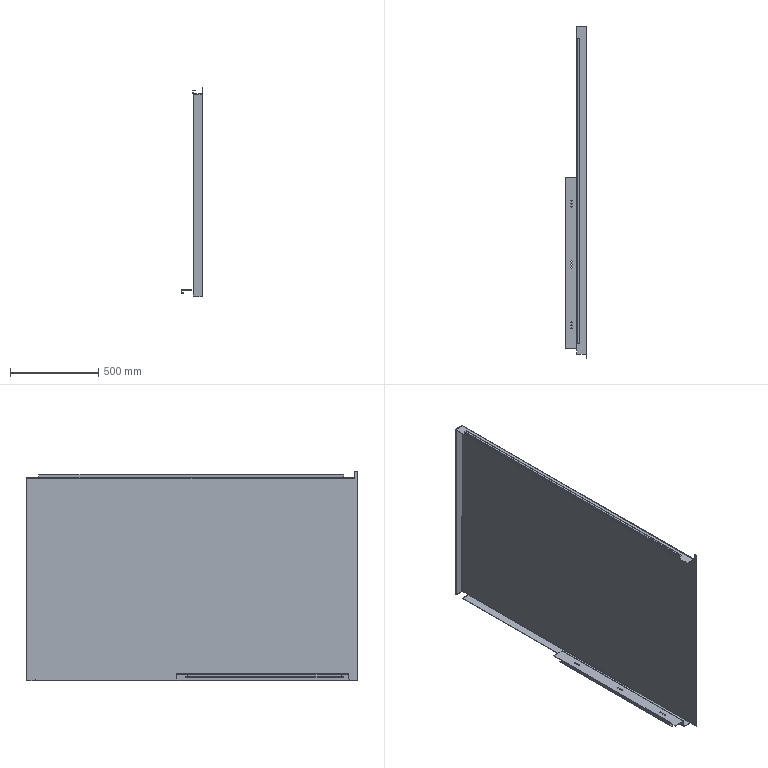Part | SolidWorks | features BaseBody 1 | 1 solid | 177 faces | box 122 x 1878 x 1185 mm | volume 5165587 mm3 | plane 153 | cylinder 20 | torus 4 | commonest cylinder face diameters 2 x9 6 x9 30 x2